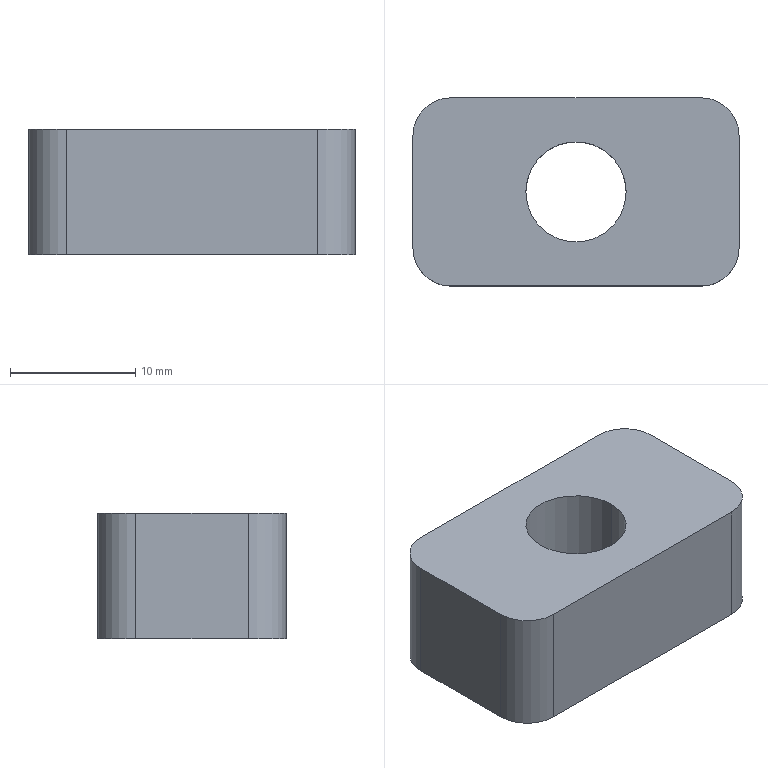Part | SolidWorks | features Extrusion 1, Fillet 1 | 1 solid | 12 faces | box 26 x 15 x 10 mm | volume 3320 mm3 | cylinder 6 | plane 6 | commonest cylinder face diameters 6 x4 8 x2
STEP:
#1=CARTESIAN_POINT('',(-4.,0.,10.));
#2=VERTEX_POINT('',#1);
#3=CARTESIAN_POINT('',(4.,0.,10.));
#4=VERTEX_POINT('',#3);
#5=CARTESIAN_POINT('',(0.,0.,10.));
#6=DIRECTION('',(0.,0.,1.));
#7=DIRECTION('',(1.,0.,0.));
#8=AXIS2_PLACEMENT_3D('',#5,#6,#7);
#9=CIRCLE('',#8,4.);
#10=EDGE_CURVE('',#2,#4,#9,.T.);
#11=ORIENTED_EDGE('',*,*,#10,.T.);
#12=CARTESIAN_POINT('',(4.,0.,0.));
#13=VERTEX_POINT('',#12);
#14=CARTESIAN_POINT('',(4.,0.,10.));
#15=DIRECTION('',(0.,0.,-1.));
#16=VECTOR('',#15,1000.);
#17=LINE('',#14,#16);
#18=EDGE_CURVE('',#4,#13,#17,.T.);
#19=ORIENTED_EDGE('',*,*,#18,.T.);
#20=CARTESIAN_POINT('',(-4.,0.,0.));
#21=VERTEX_POINT('',#20);
#22=CARTESIAN_POINT('',(0.,0.,0.));
#23=DIRECTION('',(0.,0.,1.));
#24=DIRECTION('',(1.,0.,0.));
#25=AXIS2_PLACEMENT_3D('',#22,#23,#24);
#26=CIRCLE('',#25,4.);
#27=EDGE_CURVE('',#21,#13,#26,.T.);
#28=ORIENTED_EDGE('',*,*,#27,.F.);
#29=CARTESIAN_POINT('',(-4.,0.,10.));
#30=DIRECTION('',(0.,0.,-1.));
#31=VECTOR('',#30,1000.);
#32=LINE('',#29,#31);
#33=EDGE_CURVE('',#2,#21,#32,.T.);
#34=ORIENTED_EDGE('',*,*,#33,.F.);
#35=EDGE_LOOP('',(#11,#19,#28,#34));
#36=FACE_OUTER_BOUND('',#35,.T.);
#37=CARTESIAN_POINT('',(0.,0.,10.));
#38=DIRECTION('',(0.,0.,-1.));
#39=DIRECTION('',(-1.,0.,0.));
#40=AXIS2_PLACEMENT_3D('',#37,#38,#39);
#41=CYLINDRICAL_SURFACE('',#40,4.);
#42=ADVANCED_FACE('',(#36),#41,.F.);
#43=CARTESIAN_POINT('',(10.,7.5,10.));
#44=VERTEX_POINT('',#43);
#45=CARTESIAN_POINT('',(-10.,7.5,10.));
#46=VERTEX_POINT('',#45);
#47=CARTESIAN_POINT('',(-13.,7.5,10.));
#48=DIRECTION('',(-1.,0.,0.));
#49=VECTOR('',#48,1000.);
#50=LINE('',#47,#49);
#51=EDGE_CURVE('',#44,#46,#50,.T.);
#52=ORIENTED_EDGE('',*,*,#51,.T.);
#53=CARTESIAN_POINT('',(-13.,4.5,10.));
#54=VERTEX_POINT('',#53);
#55=CARTESIAN_POINT('',(-10.,4.5,10.));
#56=DIRECTION('',(0.,0.,1.));
#57=DIRECTION('',(1.,0.,0.));
#58=AXIS2_PLACEMENT_3D('',#55,#56,#57);
#59=CIRCLE('',#58,3.);
#60=EDGE_CURVE('',#46,#54,#59,.T.);
#61=ORIENTED_EDGE('',*,*,#60,.T.);
#62=CARTESIAN_POINT('',(-13.,-4.5,10.));
#63=VERTEX_POINT('',#62);
#64=CARTESIAN_POINT('',(-13.,7.5,10.));
#65=DIRECTION('',(0.,-1.,0.));
#66=VECTOR('',#65,1000.);
#67=LINE('',#64,#66);
#68=EDGE_CURVE('',#54,#63,#67,.T.);
#69=ORIENTED_EDGE('',*,*,#68,.T.);
#70=CARTESIAN_POINT('',(-10.,-7.5,10.));
#71=VERTEX_POINT('',#70);
#72=CARTESIAN_POINT('',(-10.,-4.5,10.));
#73=DIRECTION('',(0.,0.,1.));
#74=DIRECTION('',(1.,0.,0.));
#75=AXIS2_PLACEMENT_3D('',#72,#73,#74);
#76=CIRCLE('',#75,3.);
#77=EDGE_CURVE('',#63,#71,#76,.T.);
#78=ORIENTED_EDGE('',*,*,#77,.T.);
#79=CARTESIAN_POINT('',(10.,-7.5,10.));
#80=VERTEX_POINT('',#79);
#81=CARTESIAN_POINT('',(-13.,-7.5,10.));
#82=DIRECTION('',(1.,0.,0.));
#83=VECTOR('',#82,1000.);
#84=LINE('',#81,#83);
#85=EDGE_CURVE('',#71,#80,#84,.T.);
#86=ORIENTED_EDGE('',*,*,#85,.T.);
#87=CARTESIAN_POINT('',(13.,-4.5,10.));
#88=VERTEX_POINT('',#87);
#89=CARTESIAN_POINT('',(10.,-4.5,10.));
#90=DIRECTION('',(0.,0.,1.));
#91=DIRECTION('',(1.,0.,0.));
#92=AXIS2_PLACEMENT_3D('',#89,#90,#91);
#93=CIRCLE('',#92,3.);
#94=EDGE_CURVE('',#80,#88,#93,.T.);
#95=ORIENTED_EDGE('',*,*,#94,.T.);
#96=CARTESIAN_POINT('',(13.,4.5,10.));
#97=VERTEX_POINT('',#96);
#98=CARTESIAN_POINT('',(13.,7.5,10.));
#99=DIRECTION('',(0.,1.,0.));
#100=VECTOR('',#99,1000.);
#101=LINE('',#98,#100);
#102=EDGE_CURVE('',#88,#97,#101,.T.);
#103=ORIENTED_EDGE('',*,*,#102,.T.);
#104=CARTESIAN_POINT('',(10.,4.5,10.));
#105=DIRECTION('',(0.,0.,1.));
#106=DIRECTION('',(1.,0.,0.));
#107=AXIS2_PLACEMENT_3D('',#104,#105,#106);
#108=CIRCLE('',#107,3.);
#109=EDGE_CURVE('',#97,#44,#108,.T.);
#110=ORIENTED_EDGE('',*,*,#109,.T.);
#111=EDGE_LOOP('',(#52,#61,#69,#78,#86,#95,#103,#110));
#112=FACE_OUTER_BOUND('',#111,.T.);
#113=ORIENTED_EDGE('',*,*,#10,.F.);
#114=CARTESIAN_POINT('',(0.,0.,10.));
#115=DIRECTION('',(0.,0.,1.));
#116=DIRECTION('',(1.,0.,0.));
#117=AXIS2_PLACEMENT_3D('',#114,#115,#116);
#118=CIRCLE('',#117,4.);
#119=EDGE_CURVE('',#4,#2,#118,.T.);
#120=ORIENTED_EDGE('',*,*,#119,.F.);
#121=EDGE_LOOP('',(#113,#120));
#122=FACE_BOUND('',#121,.T.);
#123=CARTESIAN_POINT('',(0.,0.,10.));
#124=DIRECTION('',(0.,0.,1.));
#125=DIRECTION('',(1.,0.,0.));
#126=AXIS2_PLACEMENT_3D('',#123,#124,#125);
#127=PLANE('',#126);
#128=ADVANCED_FACE('',(#112,#122),#127,.T.);
#129=CARTESIAN_POINT('',(-13.,4.5,0.));
#130=VERTEX_POINT('',#129);
#131=CARTESIAN_POINT('',(-13.,-4.5,0.));
#132=VERTEX_POINT('',#131);
#133=CARTESIAN_POINT('',(-13.,7.5,0.));
#134=DIRECTION('',(0.,-1.,0.));
#135=VECTOR('',#134,1000.);
#136=LINE('',#133,#135);
#137=EDGE_CURVE('',#130,#132,#136,.T.);
#138=ORIENTED_EDGE('',*,*,#137,.F.);
#139=CARTESIAN_POINT('',(-10.,7.5,0.));
#140=VERTEX_POINT('',#139);
#141=CARTESIAN_POINT('',(-10.,4.5,0.));
#142=DIRECTION('',(0.,0.,-1.));
#143=DIRECTION('',(1.,0.,0.));
#144=AXIS2_PLACEMENT_3D('',#141,#142,#143);
#145=CIRCLE('',#144,3.);
#146=EDGE_CURVE('',#130,#140,#145,.T.);
#147=ORIENTED_EDGE('',*,*,#146,.T.);
#148=CARTESIAN_POINT('',(10.,7.5,0.));
#149=VERTEX_POINT('',#148);
#150=CARTESIAN_POINT('',(-13.,7.5,0.));
#151=DIRECTION('',(-1.,0.,0.));
#152=VECTOR('',#151,1000.);
#153=LINE('',#150,#152);
#154=EDGE_CURVE('',#149,#140,#153,.T.);
#155=ORIENTED_EDGE('',*,*,#154,.F.);
#156=CARTESIAN_POINT('',(13.,4.5,0.));
#157=VERTEX_POINT('',#156);
#158=CARTESIAN_POINT('',(10.,4.5,0.));
#159=DIRECTION('',(0.,0.,-1.));
#160=DIRECTION('',(1.,0.,0.));
#161=AXIS2_PLACEMENT_3D('',#158,#159,#160);
#162=CIRCLE('',#161,3.);
#163=EDGE_CURVE('',#149,#157,#162,.T.);
#164=ORIENTED_EDGE('',*,*,#163,.T.);
#165=CARTESIAN_POINT('',(13.,-4.5,0.));
#166=VERTEX_POINT('',#165);
#167=CARTESIAN_POINT('',(13.,7.5,0.));
#168=DIRECTION('',(0.,1.,0.));
#169=VECTOR('',#168,1000.);
#170=LINE('',#167,#169);
#171=EDGE_CURVE('',#166,#157,#170,.T.);
#172=ORIENTED_EDGE('',*,*,#171,.F.);
#173=CARTESIAN_POINT('',(10.,-7.5,0.));
#174=VERTEX_POINT('',#173);
#175=CARTESIAN_POINT('',(10.,-4.5,0.));
#176=DIRECTION('',(0.,0.,-1.));
#177=DIRECTION('',(1.,0.,0.));
#178=AXIS2_PLACEMENT_3D('',#175,#176,#177);
#179=CIRCLE('',#178,3.);
#180=EDGE_CURVE('',#166,#174,#179,.T.);
#181=ORIENTED_EDGE('',*,*,#180,.T.);
#182=CARTESIAN_POINT('',(-10.,-7.5,0.));
#183=VERTEX_POINT('',#182);
#184=CARTESIAN_POINT('',(-13.,-7.5,0.));
#185=DIRECTION('',(1.,0.,0.));
#186=VECTOR('',#185,1000.);
#187=LINE('',#184,#186);
#188=EDGE_CURVE('',#183,#174,#187,.T.);
#189=ORIENTED_EDGE('',*,*,#188,.F.);
#190=CARTESIAN_POINT('',(-10.,-4.5,0.));
#191=DIRECTION('',(0.,0.,-1.));
#192=DIRECTION('',(1.,0.,0.));
#193=AXIS2_PLACEMENT_3D('',#190,#191,#192);
#194=CIRCLE('',#193,3.);
#195=EDGE_CURVE('',#183,#132,#194,.T.);
#196=ORIENTED_EDGE('',*,*,#195,.T.);
#197=EDGE_LOOP('',(#138,#147,#155,#164,#172,#181,#189,#196));
#198=FACE_OUTER_BOUND('',#197,.T.);
#199=ORIENTED_EDGE('',*,*,#27,.T.);
#200=CARTESIAN_POINT('',(0.,0.,0.));
#201=DIRECTION('',(0.,0.,1.));
#202=DIRECTION('',(1.,0.,0.));
#203=AXIS2_PLACEMENT_3D('',#200,#201,#202);
#204=CIRCLE('',#203,4.);
#205=EDGE_CURVE('',#13,#21,#204,.T.);
#206=ORIENTED_EDGE('',*,*,#205,.T.);
#207=EDGE_LOOP('',(#199,#206));
#208=FACE_BOUND('',#207,.T.);
#209=CARTESIAN_POINT('',(0.,0.,0.));
#210=DIRECTION('',(0.,0.,1.));
#211=DIRECTION('',(1.,0.,0.));
#212=AXIS2_PLACEMENT_3D('',#209,#210,#211);
#213=PLANE('',#212);
#214=ADVANCED_FACE('',(#198,#208),#213,.F.);
#215=ORIENTED_EDGE('',*,*,#102,.F.);
#216=CARTESIAN_POINT('',(13.,-4.5,10.));
#217=DIRECTION('',(0.,0.,-1.));
#218=VECTOR('',#217,1000.);
#219=LINE('',#216,#218);
#220=EDGE_CURVE('',#88,#166,#219,.T.);
#221=ORIENTED_EDGE('',*,*,#220,.T.);
#222=ORIENTED_EDGE('',*,*,#171,.T.);
#223=CARTESIAN_POINT('',(13.,4.5,10.));
#224=DIRECTION('',(0.,0.,1.));
#225=VECTOR('',#224,1000.);
#226=LINE('',#223,#225);
#227=EDGE_CURVE('',#157,#97,#226,.T.);
#228=ORIENTED_EDGE('',*,*,#227,.T.);
#229=EDGE_LOOP('',(#215,#221,#222,#228));
#230=FACE_OUTER_BOUND('',#229,.T.);
#231=CARTESIAN_POINT('',(13.,7.5,10.));
#232=DIRECTION('',(-1.,0.,0.));
#233=DIRECTION('',(0.,0.,1.));
#234=AXIS2_PLACEMENT_3D('',#231,#232,#233);
#235=PLANE('',#234);
#236=ADVANCED_FACE('',(#230),#235,.F.);
#237=ORIENTED_EDGE('',*,*,#154,.T.);
#238=CARTESIAN_POINT('',(-10.,7.5,10.));
#239=DIRECTION('',(0.,0.,1.));
#240=VECTOR('',#239,1000.);
#241=LINE('',#238,#240);
#242=EDGE_CURVE('',#140,#46,#241,.T.);
#243=ORIENTED_EDGE('',*,*,#242,.T.);
#244=ORIENTED_EDGE('',*,*,#51,.F.);
#245=CARTESIAN_POINT('',(10.,7.5,10.));
#246=DIRECTION('',(0.,0.,-1.));
#247=VECTOR('',#246,1000.);
#248=LINE('',#245,#247);
#249=EDGE_CURVE('',#44,#149,#248,.T.);
#250=ORIENTED_EDGE('',*,*,#249,.T.);
#251=EDGE_LOOP('',(#237,#243,#244,#250));
#252=FACE_OUTER_BOUND('',#251,.T.);
#253=CARTESIAN_POINT('',(-13.,7.5,10.));
#254=DIRECTION('',(0.,-1.,0.));
#255=DIRECTION('',(0.,0.,-1.));
#256=AXIS2_PLACEMENT_3D('',#253,#254,#255);
#257=PLANE('',#256);
#258=ADVANCED_FACE('',(#252),#257,.F.);
#259=ORIENTED_EDGE('',*,*,#68,.F.);
#260=CARTESIAN_POINT('',(-13.,4.5,10.));
#261=DIRECTION('',(0.,0.,-1.));
#262=VECTOR('',#261,1000.);
#263=LINE('',#260,#262);
#264=EDGE_CURVE('',#54,#130,#263,.T.);
#265=ORIENTED_EDGE('',*,*,#264,.T.);
#266=ORIENTED_EDGE('',*,*,#137,.T.);
#267=CARTESIAN_POINT('',(-13.,-4.5,10.));
#268=DIRECTION('',(0.,0.,1.));
#269=VECTOR('',#268,1000.);
#270=LINE('',#267,#269);
#271=EDGE_CURVE('',#132,#63,#270,.T.);
#272=ORIENTED_EDGE('',*,*,#271,.T.);
#273=EDGE_LOOP('',(#259,#265,#266,#272));
#274=FACE_OUTER_BOUND('',#273,.T.);
#275=CARTESIAN_POINT('',(-13.,7.5,10.));
#276=DIRECTION('',(1.,0.,0.));
#277=DIRECTION('',(0.,1.,0.));
#278=AXIS2_PLACEMENT_3D('',#275,#276,#277);
#279=PLANE('',#278);
#280=ADVANCED_FACE('',(#274),#279,.F.);
#281=ORIENTED_EDGE('',*,*,#85,.F.);
#282=CARTESIAN_POINT('',(-10.,-7.5,10.));
#283=DIRECTION('',(0.,0.,-1.));
#284=VECTOR('',#283,1000.);
#285=LINE('',#282,#284);
#286=EDGE_CURVE('',#71,#183,#285,.T.);
#287=ORIENTED_EDGE('',*,*,#286,.T.);
#288=ORIENTED_EDGE('',*,*,#188,.T.);
#289=CARTESIAN_POINT('',(10.,-7.5,10.));
#290=DIRECTION('',(0.,0.,1.));
#291=VECTOR('',#290,1000.);
#292=LINE('',#289,#291);
#293=EDGE_CURVE('',#174,#80,#292,.T.);
#294=ORIENTED_EDGE('',*,*,#293,.T.);
#295=EDGE_LOOP('',(#281,#287,#288,#294));
#296=FACE_OUTER_BOUND('',#295,.T.);
#297=CARTESIAN_POINT('',(-13.,-7.5,10.));
#298=DIRECTION('',(0.,1.,0.));
#299=DIRECTION('',(0.,0.,1.));
#300=AXIS2_PLACEMENT_3D('',#297,#298,#299);
#301=PLANE('',#300);
#302=ADVANCED_FACE('',(#296),#301,.F.);
#303=ORIENTED_EDGE('',*,*,#18,.F.);
#304=ORIENTED_EDGE('',*,*,#119,.T.);
#305=ORIENTED_EDGE('',*,*,#33,.T.);
#306=ORIENTED_EDGE('',*,*,#205,.F.);
#307=EDGE_LOOP('',(#303,#304,#305,#306));
#308=FACE_OUTER_BOUND('',#307,.T.);
#309=CARTESIAN_POINT('',(0.,0.,10.));
#310=DIRECTION('',(0.,0.,-1.));
#311=DIRECTION('',(-1.,0.,0.));
#312=AXIS2_PLACEMENT_3D('',#309,#310,#311);
#313=CYLINDRICAL_SURFACE('',#312,4.);
#314=ADVANCED_FACE('',(#308),#313,.F.);
#315=ORIENTED_EDGE('',*,*,#60,.F.);
#316=ORIENTED_EDGE('',*,*,#242,.F.);
#317=ORIENTED_EDGE('',*,*,#146,.F.);
#318=ORIENTED_EDGE('',*,*,#264,.F.);
#319=EDGE_LOOP('',(#315,#316,#317,#318));
#320=FACE_OUTER_BOUND('',#319,.T.);
#321=CARTESIAN_POINT('',(-10.,4.5,10.));
#322=DIRECTION('',(0.,0.,-1.));
#323=DIRECTION('',(-1.,0.,0.));
#324=AXIS2_PLACEMENT_3D('',#321,#322,#323);
#325=CYLINDRICAL_SURFACE('',#324,3.);
#326=ADVANCED_FACE('',(#320),#325,.T.);
#327=ORIENTED_EDGE('',*,*,#77,.F.);
#328=ORIENTED_EDGE('',*,*,#271,.F.);
#329=ORIENTED_EDGE('',*,*,#195,.F.);
#330=ORIENTED_EDGE('',*,*,#286,.F.);
#331=EDGE_LOOP('',(#327,#328,#329,#330));
#332=FACE_OUTER_BOUND('',#331,.T.);
#333=CARTESIAN_POINT('',(-10.,-4.5,10.));
#334=DIRECTION('',(0.,0.,-1.));
#335=DIRECTION('',(-1.,0.,0.));
#336=AXIS2_PLACEMENT_3D('',#333,#334,#335);
#337=CYLINDRICAL_SURFACE('',#336,3.);
#338=ADVANCED_FACE('',(#332),#337,.T.);
#339=ORIENTED_EDGE('',*,*,#94,.F.);
#340=ORIENTED_EDGE('',*,*,#293,.F.);
#341=ORIENTED_EDGE('',*,*,#180,.F.);
#342=ORIENTED_EDGE('',*,*,#220,.F.);
#343=EDGE_LOOP('',(#339,#340,#341,#342));
#344=FACE_OUTER_BOUND('',#343,.T.);
#345=CARTESIAN_POINT('',(10.,-4.5,10.));
#346=DIRECTION('',(0.,0.,-1.));
#347=DIRECTION('',(-1.,0.,0.));
#348=AXIS2_PLACEMENT_3D('',#345,#346,#347);
#349=CYLINDRICAL_SURFACE('',#348,3.);
#350=ADVANCED_FACE('',(#344),#349,.T.);
#351=ORIENTED_EDGE('',*,*,#109,.F.);
#352=ORIENTED_EDGE('',*,*,#227,.F.);
#353=ORIENTED_EDGE('',*,*,#163,.F.);
#354=ORIENTED_EDGE('',*,*,#249,.F.);
#355=EDGE_LOOP('',(#351,#352,#353,#354));
#356=FACE_OUTER_BOUND('',#355,.T.);
#357=CARTESIAN_POINT('',(10.,4.5,10.));
#358=DIRECTION('',(0.,0.,-1.));
#359=DIRECTION('',(-1.,0.,0.));
#360=AXIS2_PLACEMENT_3D('',#357,#358,#359);
#361=CYLINDRICAL_SURFACE('',#360,3.);
#362=ADVANCED_FACE('',(#356),#361,.T.);
#363=CLOSED_SHELL('',(#42,#128,#214,#236,#258,#280,#302,#314,#326,#338,#350,#362));
#364=MANIFOLD_SOLID_BREP('',#363);
#365=CARTESIAN_POINT('',(0.,0.,0.));
#366=DIRECTION('',(0.,0.,1.));
#367=DIRECTION('',(1.,0.,0.));
#368=AXIS2_PLACEMENT_3D('',#365,#366,#367);
#369=(LENGTH_UNIT()NAMED_UNIT(*)SI_UNIT(.MILLI.,.METRE.));
#370=UNCERTAINTY_MEASURE_WITH_UNIT(LENGTH_MEASURE(0.00001),#369,'','');
#371=(NAMED_UNIT(*)PLANE_ANGLE_UNIT()SI_UNIT($,.RADIAN.));
#372=(NAMED_UNIT(*)SI_UNIT($,.STERADIAN.)SOLID_ANGLE_UNIT());
#373=(GEOMETRIC_REPRESENTATION_CONTEXT(3)GLOBAL_UNCERTAINTY_ASSIGNED_CONTEXT((#370))GLOBAL_UNIT_ASSIGNED_CONTEXT((#369,#371,#372))REPRESENTATION_CONTEXT('',''));
#374=ADVANCED_BREP_SHAPE_REPRESENTATION('',(#364,#368),#373);